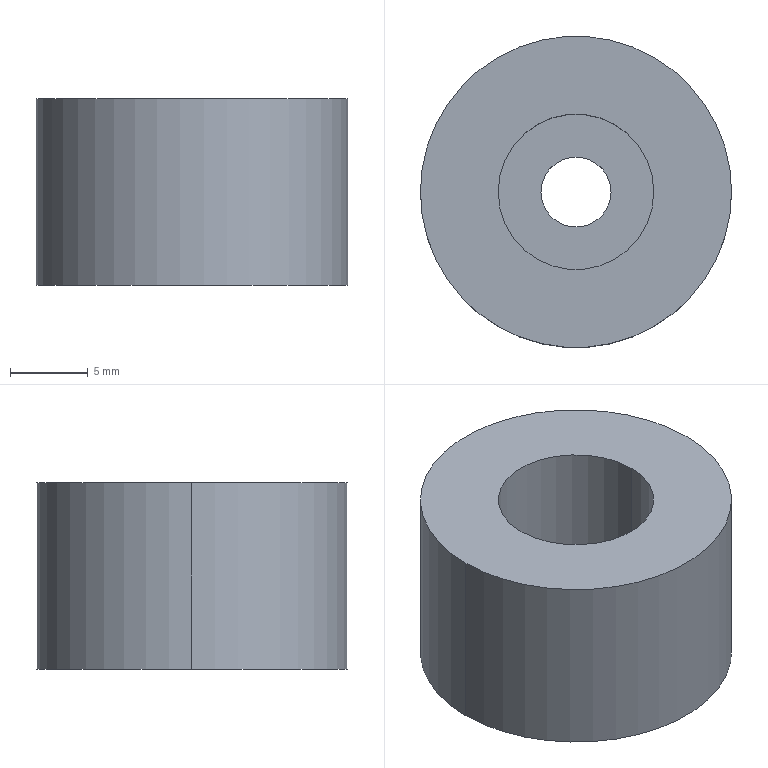Part | NX | features BREP 1 | 1 solid | 9 faces | box 20 x 20 x 12 mm | volume 3078 mm3 | cylinder 6 | plane 3 | commonest cylinder face diameters 4.5 x2 10 x2 20 x2
STEP:
#1=CARTESIAN_POINT('',(-5.,0.,12.));
#2=VERTEX_POINT('',#1);
#3=CARTESIAN_POINT('',(-5.,0.,4.));
#4=VERTEX_POINT('',#3);
#5=CARTESIAN_POINT('',(-5.,0.,12.));
#6=DIRECTION('',(0.,0.,1.));
#7=VECTOR('',#6,1000.);
#8=LINE('',#5,#7);
#9=EDGE_CURVE('',#2,#4,#8,.F.);
#10=ORIENTED_EDGE('',*,*,#9,.T.);
#11=CARTESIAN_POINT('',(5.,0.,4.));
#12=VERTEX_POINT('',#11);
#13=CARTESIAN_POINT('',(0.,0.,4.));
#14=DIRECTION('',(0.,0.,1.));
#15=DIRECTION('',(1.,0.,0.));
#16=AXIS2_PLACEMENT_3D('',#13,#14,#15);
#17=CIRCLE('',#16,5.);
#18=EDGE_CURVE('',#12,#4,#17,.T.);
#19=ORIENTED_EDGE('',*,*,#18,.F.);
#20=CARTESIAN_POINT('',(5.,0.,12.));
#21=VERTEX_POINT('',#20);
#22=CARTESIAN_POINT('',(5.,0.,12.));
#23=DIRECTION('',(0.,0.,1.));
#24=VECTOR('',#23,1000.);
#25=LINE('',#22,#24);
#26=EDGE_CURVE('',#21,#12,#25,.F.);
#27=ORIENTED_EDGE('',*,*,#26,.F.);
#28=CARTESIAN_POINT('',(0.,0.,12.));
#29=DIRECTION('',(0.,0.,1.));
#30=DIRECTION('',(1.,0.,0.));
#31=AXIS2_PLACEMENT_3D('',#28,#29,#30);
#32=CIRCLE('',#31,5.);
#33=EDGE_CURVE('',#21,#2,#32,.T.);
#34=ORIENTED_EDGE('',*,*,#33,.T.);
#35=EDGE_LOOP('',(#10,#19,#27,#34));
#36=FACE_BOUND('',#35,.T.);
#37=CARTESIAN_POINT('',(0.,0.,12.));
#38=DIRECTION('',(0.,0.,1.));
#39=DIRECTION('',(1.,0.,0.));
#40=AXIS2_PLACEMENT_3D('',#37,#38,#39);
#41=CYLINDRICAL_SURFACE('',#40,5.);
#42=ADVANCED_FACE('',(#36),#41,.F.);
#43=ORIENTED_EDGE('',*,*,#18,.T.);
#44=CARTESIAN_POINT('',(0.,0.,4.));
#45=DIRECTION('',(0.,0.,1.));
#46=DIRECTION('',(1.,0.,0.));
#47=AXIS2_PLACEMENT_3D('',#44,#45,#46);
#48=CIRCLE('',#47,5.);
#49=EDGE_CURVE('',#4,#12,#48,.T.);
#50=ORIENTED_EDGE('',*,*,#49,.T.);
#51=EDGE_LOOP('',(#43,#50));
#52=FACE_BOUND('',#51,.T.);
#53=CARTESIAN_POINT('',(2.25,0.,4.));
#54=VERTEX_POINT('',#53);
#55=CARTESIAN_POINT('',(-2.25,0.,4.));
#56=VERTEX_POINT('',#55);
#57=CARTESIAN_POINT('',(0.,0.,4.));
#58=DIRECTION('',(0.,0.,1.));
#59=DIRECTION('',(1.,0.,0.));
#60=AXIS2_PLACEMENT_3D('',#57,#58,#59);
#61=CIRCLE('',#60,2.25);
#62=EDGE_CURVE('',#54,#56,#61,.T.);
#63=ORIENTED_EDGE('',*,*,#62,.F.);
#64=CARTESIAN_POINT('',(0.,0.,4.));
#65=DIRECTION('',(0.,0.,1.));
#66=DIRECTION('',(1.,0.,0.));
#67=AXIS2_PLACEMENT_3D('',#64,#65,#66);
#68=CIRCLE('',#67,2.25);
#69=EDGE_CURVE('',#56,#54,#68,.T.);
#70=ORIENTED_EDGE('',*,*,#69,.F.);
#71=EDGE_LOOP('',(#63,#70));
#72=FACE_BOUND('',#71,.T.);
#73=CARTESIAN_POINT('',(2.25,0.,4.));
#74=DIRECTION('',(0.,0.,-1.));
#75=DIRECTION('',(-1.,0.,0.));
#76=AXIS2_PLACEMENT_3D('',#73,#74,#75);
#77=PLANE('',#76);
#78=ADVANCED_FACE('',(#52,#72),#77,.F.);
#79=CARTESIAN_POINT('',(-2.25,0.,0.));
#80=VERTEX_POINT('',#79);
#81=CARTESIAN_POINT('',(-2.25,0.,12.));
#82=DIRECTION('',(0.,0.,1.));
#83=VECTOR('',#82,1000.);
#84=LINE('',#81,#83);
#85=EDGE_CURVE('',#56,#80,#84,.F.);
#86=ORIENTED_EDGE('',*,*,#85,.T.);
#87=CARTESIAN_POINT('',(2.25,0.,0.));
#88=VERTEX_POINT('',#87);
#89=CARTESIAN_POINT('',(0.,0.,0.));
#90=DIRECTION('',(0.,0.,1.));
#91=DIRECTION('',(1.,0.,0.));
#92=AXIS2_PLACEMENT_3D('',#89,#90,#91);
#93=CIRCLE('',#92,2.25);
#94=EDGE_CURVE('',#88,#80,#93,.T.);
#95=ORIENTED_EDGE('',*,*,#94,.F.);
#96=CARTESIAN_POINT('',(2.25,0.,12.));
#97=DIRECTION('',(0.,0.,1.));
#98=VECTOR('',#97,1000.);
#99=LINE('',#96,#98);
#100=EDGE_CURVE('',#54,#88,#99,.F.);
#101=ORIENTED_EDGE('',*,*,#100,.F.);
#102=ORIENTED_EDGE('',*,*,#62,.T.);
#103=EDGE_LOOP('',(#86,#95,#101,#102));
#104=FACE_BOUND('',#103,.T.);
#105=CARTESIAN_POINT('',(0.,0.,12.));
#106=DIRECTION('',(0.,0.,1.));
#107=DIRECTION('',(1.,0.,0.));
#108=AXIS2_PLACEMENT_3D('',#105,#106,#107);
#109=CYLINDRICAL_SURFACE('',#108,2.25);
#110=ADVANCED_FACE('',(#104),#109,.F.);
#111=CARTESIAN_POINT('',(-10.,0.,0.));
#112=VERTEX_POINT('',#111);
#113=CARTESIAN_POINT('',(10.,0.,0.));
#114=VERTEX_POINT('',#113);
#115=CARTESIAN_POINT('',(0.,0.,0.));
#116=DIRECTION('',(0.,0.,1.));
#117=DIRECTION('',(1.,0.,0.));
#118=AXIS2_PLACEMENT_3D('',#115,#116,#117);
#119=CIRCLE('',#118,10.);
#120=EDGE_CURVE('',#112,#114,#119,.T.);
#121=ORIENTED_EDGE('',*,*,#120,.F.);
#122=CARTESIAN_POINT('',(0.,0.,0.));
#123=DIRECTION('',(0.,0.,1.));
#124=DIRECTION('',(1.,0.,0.));
#125=AXIS2_PLACEMENT_3D('',#122,#123,#124);
#126=CIRCLE('',#125,10.);
#127=EDGE_CURVE('',#114,#112,#126,.T.);
#128=ORIENTED_EDGE('',*,*,#127,.F.);
#129=EDGE_LOOP('',(#121,#128));
#130=FACE_BOUND('',#129,.T.);
#131=ORIENTED_EDGE('',*,*,#94,.T.);
#132=CARTESIAN_POINT('',(0.,0.,0.));
#133=DIRECTION('',(0.,0.,1.));
#134=DIRECTION('',(1.,0.,0.));
#135=AXIS2_PLACEMENT_3D('',#132,#133,#134);
#136=CIRCLE('',#135,2.25);
#137=EDGE_CURVE('',#80,#88,#136,.T.);
#138=ORIENTED_EDGE('',*,*,#137,.T.);
#139=EDGE_LOOP('',(#131,#138));
#140=FACE_BOUND('',#139,.T.);
#141=CARTESIAN_POINT('',(0.,0.,0.));
#142=DIRECTION('',(0.,0.,1.));
#143=DIRECTION('',(1.,0.,0.));
#144=AXIS2_PLACEMENT_3D('',#141,#142,#143);
#145=PLANE('',#144);
#146=ADVANCED_FACE('',(#130,#140),#145,.F.);
#147=CARTESIAN_POINT('',(-10.,0.,12.));
#148=VERTEX_POINT('',#147);
#149=CARTESIAN_POINT('',(10.,0.,12.));
#150=VERTEX_POINT('',#149);
#151=CARTESIAN_POINT('',(0.,0.,12.));
#152=DIRECTION('',(0.,0.,1.));
#153=DIRECTION('',(1.,0.,0.));
#154=AXIS2_PLACEMENT_3D('',#151,#152,#153);
#155=CIRCLE('',#154,10.);
#156=EDGE_CURVE('',#148,#150,#155,.T.);
#157=ORIENTED_EDGE('',*,*,#156,.T.);
#158=CARTESIAN_POINT('',(0.,0.,12.));
#159=DIRECTION('',(0.,0.,1.));
#160=DIRECTION('',(1.,0.,0.));
#161=AXIS2_PLACEMENT_3D('',#158,#159,#160);
#162=CIRCLE('',#161,10.);
#163=EDGE_CURVE('',#150,#148,#162,.T.);
#164=ORIENTED_EDGE('',*,*,#163,.T.);
#165=EDGE_LOOP('',(#157,#164));
#166=FACE_BOUND('',#165,.T.);
#167=ORIENTED_EDGE('',*,*,#33,.F.);
#168=CARTESIAN_POINT('',(0.,0.,12.));
#169=DIRECTION('',(0.,0.,1.));
#170=DIRECTION('',(1.,0.,0.));
#171=AXIS2_PLACEMENT_3D('',#168,#169,#170);
#172=CIRCLE('',#171,5.);
#173=EDGE_CURVE('',#2,#21,#172,.T.);
#174=ORIENTED_EDGE('',*,*,#173,.F.);
#175=EDGE_LOOP('',(#167,#174));
#176=FACE_BOUND('',#175,.T.);
#177=CARTESIAN_POINT('',(0.,0.,12.));
#178=DIRECTION('',(0.,0.,1.));
#179=DIRECTION('',(1.,0.,0.));
#180=AXIS2_PLACEMENT_3D('',#177,#178,#179);
#181=PLANE('',#180);
#182=ADVANCED_FACE('',(#166,#176),#181,.T.);
#183=CARTESIAN_POINT('',(10.,0.,12.));
#184=DIRECTION('',(0.,0.,-1.));
#185=VECTOR('',#184,1000.);
#186=LINE('',#183,#185);
#187=EDGE_CURVE('',#150,#114,#186,.T.);
#188=ORIENTED_EDGE('',*,*,#187,.F.);
#189=ORIENTED_EDGE('',*,*,#156,.F.);
#190=CARTESIAN_POINT('',(-10.,0.,12.));
#191=DIRECTION('',(0.,0.,-1.));
#192=VECTOR('',#191,1000.);
#193=LINE('',#190,#192);
#194=EDGE_CURVE('',#148,#112,#193,.T.);
#195=ORIENTED_EDGE('',*,*,#194,.T.);
#196=ORIENTED_EDGE('',*,*,#120,.T.);
#197=EDGE_LOOP('',(#188,#189,#195,#196));
#198=FACE_BOUND('',#197,.T.);
#199=CARTESIAN_POINT('',(0.,0.,12.));
#200=DIRECTION('',(0.,0.,-1.));
#201=DIRECTION('',(-1.,0.,0.));
#202=AXIS2_PLACEMENT_3D('',#199,#200,#201);
#203=CYLINDRICAL_SURFACE('',#202,10.);
#204=ADVANCED_FACE('',(#198),#203,.T.);
#205=ORIENTED_EDGE('',*,*,#163,.F.);
#206=ORIENTED_EDGE('',*,*,#187,.T.);
#207=ORIENTED_EDGE('',*,*,#127,.T.);
#208=ORIENTED_EDGE('',*,*,#194,.F.);
#209=EDGE_LOOP('',(#205,#206,#207,#208));
#210=FACE_BOUND('',#209,.T.);
#211=CARTESIAN_POINT('',(0.,0.,12.));
#212=DIRECTION('',(0.,0.,-1.));
#213=DIRECTION('',(-1.,0.,0.));
#214=AXIS2_PLACEMENT_3D('',#211,#212,#213);
#215=CYLINDRICAL_SURFACE('',#214,10.);
#216=ADVANCED_FACE('',(#210),#215,.T.);
#217=ORIENTED_EDGE('',*,*,#137,.F.);
#218=ORIENTED_EDGE('',*,*,#85,.F.);
#219=ORIENTED_EDGE('',*,*,#69,.T.);
#220=ORIENTED_EDGE('',*,*,#100,.T.);
#221=EDGE_LOOP('',(#217,#218,#219,#220));
#222=FACE_BOUND('',#221,.T.);
#223=CARTESIAN_POINT('',(0.,0.,12.));
#224=DIRECTION('',(0.,0.,1.));
#225=DIRECTION('',(1.,0.,0.));
#226=AXIS2_PLACEMENT_3D('',#223,#224,#225);
#227=CYLINDRICAL_SURFACE('',#226,2.25);
#228=ADVANCED_FACE('',(#222),#227,.F.);
#229=ORIENTED_EDGE('',*,*,#49,.F.);
#230=ORIENTED_EDGE('',*,*,#9,.F.);
#231=ORIENTED_EDGE('',*,*,#173,.T.);
#232=ORIENTED_EDGE('',*,*,#26,.T.);
#233=EDGE_LOOP('',(#229,#230,#231,#232));
#234=FACE_BOUND('',#233,.T.);
#235=CARTESIAN_POINT('',(0.,0.,12.));
#236=DIRECTION('',(0.,0.,1.));
#237=DIRECTION('',(1.,0.,0.));
#238=AXIS2_PLACEMENT_3D('',#235,#236,#237);
#239=CYLINDRICAL_SURFACE('',#238,5.);
#240=ADVANCED_FACE('',(#234),#239,.F.);
#241=CLOSED_SHELL('',(#42,#78,#110,#146,#182,#204,#216,#228,#240));
#242=MANIFOLD_SOLID_BREP('',#241);
#243=(LENGTH_UNIT()NAMED_UNIT(*)SI_UNIT(.MILLI.,.METRE.));
#244=UNCERTAINTY_MEASURE_WITH_UNIT(LENGTH_MEASURE(0.00001),#243,'','');
#245=(NAMED_UNIT(*)PLANE_ANGLE_UNIT()SI_UNIT($,.RADIAN.));
#246=(NAMED_UNIT(*)SI_UNIT($,.STERADIAN.)SOLID_ANGLE_UNIT());
#247=(GEOMETRIC_REPRESENTATION_CONTEXT(3)GLOBAL_UNCERTAINTY_ASSIGNED_CONTEXT((#244))GLOBAL_UNIT_ASSIGNED_CONTEXT((#243,#245,#246))REPRESENTATION_CONTEXT('',''));
#248=ADVANCED_BREP_SHAPE_REPRESENTATION('',(#242),#247);